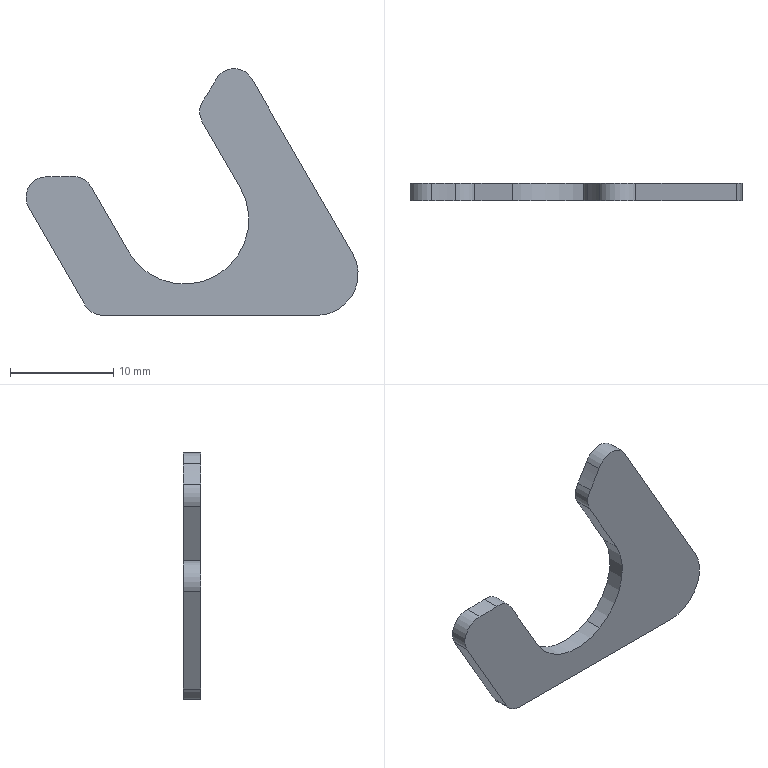Part | SolidWorks | features BaseBody 1 | 1 solid | 18 faces | box 32.238 x 1.7 x 23.947 mm | volume 539.449 mm3 | cylinder 11 | plane 7 | commonest cylinder face diameters 4 x5 8 x2 12.5 x2 35 x2
STEP:
#1=CARTESIAN_POINT('',(258.361,160.,-32.991));
#2=VERTEX_POINT('',#1);
#3=CARTESIAN_POINT('',(259.825,160.,-27.527));
#4=VERTEX_POINT('',#3);
#5=CARTESIAN_POINT('',(256.361,160.,-29.527));
#6=DIRECTION('',(0.,-1.,0.));
#7=DIRECTION('',(0.5,0.,-0.866));
#8=AXIS2_PLACEMENT_3D('',#5,#6,#7);
#9=CIRCLE('',#8,4.);
#10=EDGE_CURVE('',#2,#4,#9,.T.);
#11=ORIENTED_EDGE('',*,*,#10,.F.);
#12=CARTESIAN_POINT('',(258.361,161.7,-32.991));
#13=VERTEX_POINT('',#12);
#14=CARTESIAN_POINT('',(258.361,160.,-32.991));
#15=DIRECTION('',(0.,1.,0.));
#16=VECTOR('',#15,1000.);
#17=LINE('',#14,#16);
#18=EDGE_CURVE('',#2,#13,#17,.T.);
#19=ORIENTED_EDGE('',*,*,#18,.T.);
#20=CARTESIAN_POINT('',(259.825,161.7,-27.527));
#21=VERTEX_POINT('',#20);
#22=CARTESIAN_POINT('',(256.361,161.7,-29.527));
#23=DIRECTION('',(0.,-1.,0.));
#24=DIRECTION('',(0.5,0.,-0.866));
#25=AXIS2_PLACEMENT_3D('',#22,#23,#24);
#26=CIRCLE('',#25,4.);
#27=EDGE_CURVE('',#13,#21,#26,.T.);
#28=ORIENTED_EDGE('',*,*,#27,.T.);
#29=CARTESIAN_POINT('',(259.825,160.,-27.527));
#30=DIRECTION('',(0.,1.,0.));
#31=VECTOR('',#30,1000.);
#32=LINE('',#29,#31);
#33=EDGE_CURVE('',#4,#21,#32,.T.);
#34=ORIENTED_EDGE('',*,*,#33,.F.);
#35=EDGE_LOOP('',(#11,#19,#28,#34));
#36=FACE_OUTER_BOUND('',#35,.T.);
#37=CARTESIAN_POINT('',(256.361,160.,-29.527));
#38=DIRECTION('',(0.,1.,0.));
#39=DIRECTION('',(0.5,0.,-0.866));
#40=AXIS2_PLACEMENT_3D('',#37,#38,#39);
#41=CYLINDRICAL_SURFACE('',#40,4.);
#42=ADVANCED_FACE('',(#36),#41,.T.);
#43=CARTESIAN_POINT('',(246.625,160.,-29.663));
#44=VERTEX_POINT('',#43);
#45=CARTESIAN_POINT('',(238.087,160.,-27.375));
#46=VERTEX_POINT('',#45);
#47=CARTESIAN_POINT('',(243.5,160.,-24.25));
#48=DIRECTION('',(0.,1.,0.));
#49=DIRECTION('',(-0.5,0.,0.866));
#50=AXIS2_PLACEMENT_3D('',#47,#48,#49);
#51=CIRCLE('',#50,6.25);
#52=EDGE_CURVE('',#44,#46,#51,.T.);
#53=ORIENTED_EDGE('',*,*,#52,.F.);
#54=CARTESIAN_POINT('',(246.625,161.7,-29.663));
#55=VERTEX_POINT('',#54);
#56=CARTESIAN_POINT('',(246.625,160.,-29.663));
#57=DIRECTION('',(0.,1.,0.));
#58=VECTOR('',#57,1000.);
#59=LINE('',#56,#58);
#60=EDGE_CURVE('',#44,#55,#59,.T.);
#61=ORIENTED_EDGE('',*,*,#60,.T.);
#62=CARTESIAN_POINT('',(238.087,161.7,-27.375));
#63=VERTEX_POINT('',#62);
#64=CARTESIAN_POINT('',(243.5,161.7,-24.25));
#65=DIRECTION('',(0.,1.,0.));
#66=DIRECTION('',(-0.5,0.,0.866));
#67=AXIS2_PLACEMENT_3D('',#64,#65,#66);
#68=CIRCLE('',#67,6.25);
#69=EDGE_CURVE('',#55,#63,#68,.T.);
#70=ORIENTED_EDGE('',*,*,#69,.T.);
#71=CARTESIAN_POINT('',(238.087,160.,-27.375));
#72=DIRECTION('',(0.,1.,0.));
#73=VECTOR('',#72,1000.);
#74=LINE('',#71,#73);
#75=EDGE_CURVE('',#46,#63,#74,.T.);
#76=ORIENTED_EDGE('',*,*,#75,.F.);
#77=EDGE_LOOP('',(#53,#61,#70,#76));
#78=FACE_OUTER_BOUND('',#77,.T.);
#79=CARTESIAN_POINT('',(243.5,160.,-24.25));
#80=DIRECTION('',(0.,1.,0.));
#81=DIRECTION('',(0.5,0.,-0.866));
#82=AXIS2_PLACEMENT_3D('',#79,#80,#81);
#83=CYLINDRICAL_SURFACE('',#82,6.25);
#84=ADVANCED_FACE('',(#78),#83,.F.);
#85=ORIENTED_EDGE('',*,*,#60,.F.);
#86=CARTESIAN_POINT('',(248.913,160.,-21.125));
#87=VERTEX_POINT('',#86);
#88=CARTESIAN_POINT('',(243.5,160.,-24.25));
#89=DIRECTION('',(0.,1.,0.));
#90=DIRECTION('',(-0.5,0.,0.866));
#91=AXIS2_PLACEMENT_3D('',#88,#89,#90);
#92=CIRCLE('',#91,6.25);
#93=EDGE_CURVE('',#87,#44,#92,.T.);
#94=ORIENTED_EDGE('',*,*,#93,.F.);
#95=CARTESIAN_POINT('',(248.913,161.7,-21.125));
#96=VERTEX_POINT('',#95);
#97=CARTESIAN_POINT('',(248.913,160.,-21.125));
#98=DIRECTION('',(0.,1.,0.));
#99=VECTOR('',#98,1000.);
#100=LINE('',#97,#99);
#101=EDGE_CURVE('',#87,#96,#100,.T.);
#102=ORIENTED_EDGE('',*,*,#101,.T.);
#103=CARTESIAN_POINT('',(243.5,161.7,-24.25));
#104=DIRECTION('',(0.,1.,0.));
#105=DIRECTION('',(-0.5,0.,0.866));
#106=AXIS2_PLACEMENT_3D('',#103,#104,#105);
#107=CIRCLE('',#106,6.25);
#108=EDGE_CURVE('',#96,#55,#107,.T.);
#109=ORIENTED_EDGE('',*,*,#108,.T.);
#110=EDGE_LOOP('',(#85,#94,#102,#109));
#111=FACE_OUTER_BOUND('',#110,.T.);
#112=CARTESIAN_POINT('',(243.5,160.,-24.25));
#113=DIRECTION('',(0.,1.,0.));
#114=DIRECTION('',(0.5,0.,-0.866));
#115=AXIS2_PLACEMENT_3D('',#112,#113,#114);
#116=CYLINDRICAL_SURFACE('',#115,6.25);
#117=ADVANCED_FACE('',(#111),#116,.F.);
#118=CARTESIAN_POINT('',(234.422,161.7,-21.026));
#119=VERTEX_POINT('',#118);
#120=CARTESIAN_POINT('',(238.087,161.7,-27.375));
#121=DIRECTION('',(-0.5,0.,0.866));
#122=VECTOR('',#121,1000.);
#123=LINE('',#120,#122);
#124=EDGE_CURVE('',#63,#119,#123,.T.);
#125=ORIENTED_EDGE('',*,*,#124,.T.);
#126=CARTESIAN_POINT('',(234.422,160.,-21.026));
#127=VERTEX_POINT('',#126);
#128=CARTESIAN_POINT('',(234.422,160.,-21.026));
#129=DIRECTION('',(0.,1.,0.));
#130=VECTOR('',#129,1000.);
#131=LINE('',#128,#130);
#132=EDGE_CURVE('',#127,#119,#131,.T.);
#133=ORIENTED_EDGE('',*,*,#132,.F.);
#134=CARTESIAN_POINT('',(238.087,160.,-27.375));
#135=DIRECTION('',(-0.5,0.,0.866));
#136=VECTOR('',#135,1000.);
#137=LINE('',#134,#136);
#138=EDGE_CURVE('',#46,#127,#137,.T.);
#139=ORIENTED_EDGE('',*,*,#138,.F.);
#140=ORIENTED_EDGE('',*,*,#75,.T.);
#141=EDGE_LOOP('',(#125,#133,#139,#140));
#142=FACE_OUTER_BOUND('',#141,.T.);
#143=CARTESIAN_POINT('',(238.087,160.,-27.375));
#144=DIRECTION('',(-0.866,0.,-0.5));
#145=DIRECTION('',(0.5,0.,-0.866));
#146=AXIS2_PLACEMENT_3D('',#143,#144,#145);
#147=PLANE('',#146);
#148=ADVANCED_FACE('',(#142),#147,.F.);
#149=CARTESIAN_POINT('',(232.516,161.7,-20.033));
#150=VERTEX_POINT('',#149);
#151=CARTESIAN_POINT('',(232.69,161.7,-22.026));
#152=DIRECTION('',(0.,-1.,0.));
#153=DIRECTION('',(-0.5,0.,0.866));
#154=AXIS2_PLACEMENT_3D('',#151,#152,#153);
#155=CIRCLE('',#154,2.);
#156=EDGE_CURVE('',#119,#150,#155,.T.);
#157=ORIENTED_EDGE('',*,*,#156,.T.);
#158=CARTESIAN_POINT('',(232.516,160.,-20.033));
#159=VERTEX_POINT('',#158);
#160=CARTESIAN_POINT('',(232.516,160.,-20.033));
#161=DIRECTION('',(0.,1.,0.));
#162=VECTOR('',#161,1000.);
#163=LINE('',#160,#162);
#164=EDGE_CURVE('',#159,#150,#163,.T.);
#165=ORIENTED_EDGE('',*,*,#164,.F.);
#166=CARTESIAN_POINT('',(232.69,160.,-22.026));
#167=DIRECTION('',(0.,-1.,0.));
#168=DIRECTION('',(-0.5,0.,0.866));
#169=AXIS2_PLACEMENT_3D('',#166,#167,#168);
#170=CIRCLE('',#169,2.);
#171=EDGE_CURVE('',#127,#159,#170,.T.);
#172=ORIENTED_EDGE('',*,*,#171,.F.);
#173=ORIENTED_EDGE('',*,*,#132,.T.);
#174=EDGE_LOOP('',(#157,#165,#172,#173));
#175=FACE_OUTER_BOUND('',#174,.T.);
#176=CARTESIAN_POINT('',(232.69,160.,-22.026));
#177=DIRECTION('',(0.,1.,0.));
#178=DIRECTION('',(0.5,0.,-0.866));
#179=AXIS2_PLACEMENT_3D('',#176,#177,#178);
#180=CYLINDRICAL_SURFACE('',#179,2.);
#181=ADVANCED_FACE('',(#175),#180,.T.);
#182=CARTESIAN_POINT('',(230.213,161.7,-20.081));
#183=VERTEX_POINT('',#182);
#184=CARTESIAN_POINT('',(231.,161.7,-2.599));
#185=DIRECTION('',(0.,1.,0.));
#186=DIRECTION('',(-0.5,0.,0.866));
#187=AXIS2_PLACEMENT_3D('',#184,#185,#186);
#188=CIRCLE('',#187,17.5);
#189=EDGE_CURVE('',#150,#183,#188,.T.);
#190=ORIENTED_EDGE('',*,*,#189,.T.);
#191=CARTESIAN_POINT('',(230.213,160.,-20.081));
#192=VERTEX_POINT('',#191);
#193=CARTESIAN_POINT('',(230.213,160.,-20.081));
#194=DIRECTION('',(0.,1.,0.));
#195=VECTOR('',#194,1000.);
#196=LINE('',#193,#195);
#197=EDGE_CURVE('',#192,#183,#196,.T.);
#198=ORIENTED_EDGE('',*,*,#197,.F.);
#199=CARTESIAN_POINT('',(231.,160.,-2.599));
#200=DIRECTION('',(0.,1.,0.));
#201=DIRECTION('',(-0.5,0.,0.866));
#202=AXIS2_PLACEMENT_3D('',#199,#200,#201);
#203=CIRCLE('',#202,17.5);
#204=EDGE_CURVE('',#159,#192,#203,.T.);
#205=ORIENTED_EDGE('',*,*,#204,.F.);
#206=ORIENTED_EDGE('',*,*,#164,.T.);
#207=EDGE_LOOP('',(#190,#198,#205,#206));
#208=FACE_OUTER_BOUND('',#207,.T.);
#209=CARTESIAN_POINT('',(231.,160.,-2.599));
#210=DIRECTION('',(0.,1.,0.));
#211=DIRECTION('',(0.5,0.,-0.866));
#212=AXIS2_PLACEMENT_3D('',#209,#210,#211);
#213=CYLINDRICAL_SURFACE('',#212,17.5);
#214=ADVANCED_FACE('',(#208),#213,.F.);
#215=CARTESIAN_POINT('',(228.391,161.7,-23.079));
#216=VERTEX_POINT('',#215);
#217=CARTESIAN_POINT('',(230.123,161.7,-22.079));
#218=DIRECTION('',(0.,-1.,0.));
#219=DIRECTION('',(0.5,0.,-0.866));
#220=AXIS2_PLACEMENT_3D('',#217,#218,#219);
#221=CIRCLE('',#220,2.);
#222=EDGE_CURVE('',#183,#216,#221,.T.);
#223=ORIENTED_EDGE('',*,*,#222,.T.);
#224=CARTESIAN_POINT('',(228.391,160.,-23.079));
#225=VERTEX_POINT('',#224);
#226=CARTESIAN_POINT('',(228.391,160.,-23.079));
#227=DIRECTION('',(0.,1.,0.));
#228=VECTOR('',#227,1000.);
#229=LINE('',#226,#228);
#230=EDGE_CURVE('',#225,#216,#229,.T.);
#231=ORIENTED_EDGE('',*,*,#230,.F.);
#232=CARTESIAN_POINT('',(230.123,160.,-22.079));
#233=DIRECTION('',(0.,-1.,0.));
#234=DIRECTION('',(0.5,0.,-0.866));
#235=AXIS2_PLACEMENT_3D('',#232,#233,#234);
#236=CIRCLE('',#235,2.);
#237=EDGE_CURVE('',#192,#225,#236,.T.);
#238=ORIENTED_EDGE('',*,*,#237,.F.);
#239=ORIENTED_EDGE('',*,*,#197,.T.);
#240=EDGE_LOOP('',(#223,#231,#238,#239));
#241=FACE_OUTER_BOUND('',#240,.T.);
#242=CARTESIAN_POINT('',(230.123,160.,-22.079));
#243=DIRECTION('',(0.,1.,0.));
#244=DIRECTION('',(0.5,0.,-0.866));
#245=AXIS2_PLACEMENT_3D('',#242,#243,#244);
#246=CYLINDRICAL_SURFACE('',#245,2.);
#247=ADVANCED_FACE('',(#241),#246,.T.);
#248=CARTESIAN_POINT('',(233.844,161.7,-32.526));
#249=VERTEX_POINT('',#248);
#250=CARTESIAN_POINT('',(233.844,161.7,-32.526));
#251=DIRECTION('',(0.5,0.,-0.866));
#252=VECTOR('',#251,1000.);
#253=LINE('',#250,#252);
#254=EDGE_CURVE('',#216,#249,#253,.T.);
#255=ORIENTED_EDGE('',*,*,#254,.T.);
#256=CARTESIAN_POINT('',(233.844,160.,-32.526));
#257=VERTEX_POINT('',#256);
#258=CARTESIAN_POINT('',(233.844,160.,-32.526));
#259=DIRECTION('',(0.,1.,0.));
#260=VECTOR('',#259,1000.);
#261=LINE('',#258,#260);
#262=EDGE_CURVE('',#257,#249,#261,.T.);
#263=ORIENTED_EDGE('',*,*,#262,.F.);
#264=CARTESIAN_POINT('',(233.844,160.,-32.526));
#265=DIRECTION('',(0.5,0.,-0.866));
#266=VECTOR('',#265,1000.);
#267=LINE('',#264,#266);
#268=EDGE_CURVE('',#225,#257,#267,.T.);
#269=ORIENTED_EDGE('',*,*,#268,.F.);
#270=ORIENTED_EDGE('',*,*,#230,.T.);
#271=EDGE_LOOP('',(#255,#263,#269,#270));
#272=FACE_OUTER_BOUND('',#271,.T.);
#273=CARTESIAN_POINT('',(233.844,160.,-32.526));
#274=DIRECTION('',(0.866,0.,0.5));
#275=DIRECTION('',(-0.5,0.,0.866));
#276=AXIS2_PLACEMENT_3D('',#273,#274,#275);
#277=PLANE('',#276);
#278=ADVANCED_FACE('',(#272),#277,.F.);
#279=CARTESIAN_POINT('',(235.576,161.7,-33.526));
#280=VERTEX_POINT('',#279);
#281=CARTESIAN_POINT('',(235.576,161.7,-31.526));
#282=DIRECTION('',(0.,-1.,0.));
#283=DIRECTION('',(0.5,0.,-0.866));
#284=AXIS2_PLACEMENT_3D('',#281,#282,#283);
#285=CIRCLE('',#284,2.);
#286=EDGE_CURVE('',#249,#280,#285,.T.);
#287=ORIENTED_EDGE('',*,*,#286,.T.);
#288=CARTESIAN_POINT('',(235.576,160.,-33.526));
#289=VERTEX_POINT('',#288);
#290=CARTESIAN_POINT('',(235.576,160.,-33.526));
#291=DIRECTION('',(0.,1.,0.));
#292=VECTOR('',#291,1000.);
#293=LINE('',#290,#292);
#294=EDGE_CURVE('',#289,#280,#293,.T.);
#295=ORIENTED_EDGE('',*,*,#294,.F.);
#296=CARTESIAN_POINT('',(235.576,160.,-31.526));
#297=DIRECTION('',(0.,-1.,0.));
#298=DIRECTION('',(0.5,0.,-0.866));
#299=AXIS2_PLACEMENT_3D('',#296,#297,#298);
#300=CIRCLE('',#299,2.);
#301=EDGE_CURVE('',#257,#289,#300,.T.);
#302=ORIENTED_EDGE('',*,*,#301,.F.);
#303=ORIENTED_EDGE('',*,*,#262,.T.);
#304=EDGE_LOOP('',(#287,#295,#302,#303));
#305=FACE_OUTER_BOUND('',#304,.T.);
#306=CARTESIAN_POINT('',(235.576,160.,-31.526));
#307=DIRECTION('',(0.,1.,0.));
#308=DIRECTION('',(0.5,0.,-0.866));
#309=AXIS2_PLACEMENT_3D('',#306,#307,#308);
#310=CYLINDRICAL_SURFACE('',#309,2.);
#311=ADVANCED_FACE('',(#305),#310,.T.);
#312=CARTESIAN_POINT('',(256.361,161.7,-33.527));
#313=VERTEX_POINT('',#312);
#314=CARTESIAN_POINT('',(235.576,161.7,-33.526));
#315=DIRECTION('',(1.,0.,-0.00002301));
#316=VECTOR('',#315,1000.);
#317=LINE('',#314,#316);
#318=EDGE_CURVE('',#280,#313,#317,.T.);
#319=ORIENTED_EDGE('',*,*,#318,.T.);
#320=CARTESIAN_POINT('',(256.361,160.,-33.527));
#321=VERTEX_POINT('',#320);
#322=CARTESIAN_POINT('',(256.361,160.,-33.527));
#323=DIRECTION('',(0.,1.,0.));
#324=VECTOR('',#323,1000.);
#325=LINE('',#322,#324);
#326=EDGE_CURVE('',#321,#313,#325,.T.);
#327=ORIENTED_EDGE('',*,*,#326,.F.);
#328=CARTESIAN_POINT('',(235.576,160.,-33.526));
#329=DIRECTION('',(1.,0.,-0.00002301));
#330=VECTOR('',#329,1000.);
#331=LINE('',#328,#330);
#332=EDGE_CURVE('',#289,#321,#331,.T.);
#333=ORIENTED_EDGE('',*,*,#332,.F.);
#334=ORIENTED_EDGE('',*,*,#294,.T.);
#335=EDGE_LOOP('',(#319,#327,#333,#334));
#336=FACE_OUTER_BOUND('',#335,.T.);
#337=CARTESIAN_POINT('',(235.576,160.,-33.526));
#338=DIRECTION('',(0.00002301,0.,1.));
#339=DIRECTION('',(-1.,0.,0.00002301));
#340=AXIS2_PLACEMENT_3D('',#337,#338,#339);
#341=PLANE('',#340);
#342=ADVANCED_FACE('',(#336),#341,.F.);
#343=ORIENTED_EDGE('',*,*,#18,.F.);
#344=CARTESIAN_POINT('',(256.361,160.,-29.527));
#345=DIRECTION('',(0.,-1.,0.));
#346=DIRECTION('',(0.5,0.,-0.866));
#347=AXIS2_PLACEMENT_3D('',#344,#345,#346);
#348=CIRCLE('',#347,4.);
#349=EDGE_CURVE('',#321,#2,#348,.T.);
#350=ORIENTED_EDGE('',*,*,#349,.F.);
#351=ORIENTED_EDGE('',*,*,#326,.T.);
#352=CARTESIAN_POINT('',(256.361,161.7,-29.527));
#353=DIRECTION('',(0.,-1.,0.));
#354=DIRECTION('',(0.5,0.,-0.866));
#355=AXIS2_PLACEMENT_3D('',#352,#353,#354);
#356=CIRCLE('',#355,4.);
#357=EDGE_CURVE('',#313,#13,#356,.T.);
#358=ORIENTED_EDGE('',*,*,#357,.T.);
#359=EDGE_LOOP('',(#343,#350,#351,#358));
#360=FACE_OUTER_BOUND('',#359,.T.);
#361=CARTESIAN_POINT('',(256.361,160.,-29.527));
#362=DIRECTION('',(0.,1.,0.));
#363=DIRECTION('',(0.5,0.,-0.866));
#364=AXIS2_PLACEMENT_3D('',#361,#362,#363);
#365=CYLINDRICAL_SURFACE('',#364,4.);
#366=ADVANCED_FACE('',(#360),#365,.T.);
#367=CARTESIAN_POINT('',(250.041,161.7,-10.58));
#368=VERTEX_POINT('',#367);
#369=CARTESIAN_POINT('',(259.825,161.7,-27.527));
#370=DIRECTION('',(-0.5,0.,0.866));
#371=VECTOR('',#370,1000.);
#372=LINE('',#369,#371);
#373=EDGE_CURVE('',#21,#368,#372,.T.);
#374=ORIENTED_EDGE('',*,*,#373,.T.);
#375=CARTESIAN_POINT('',(250.041,160.,-10.58));
#376=VERTEX_POINT('',#375);
#377=CARTESIAN_POINT('',(250.041,160.,-10.58));
#378=DIRECTION('',(0.,1.,0.));
#379=VECTOR('',#378,1000.);
#380=LINE('',#377,#379);
#381=EDGE_CURVE('',#376,#368,#380,.T.);
#382=ORIENTED_EDGE('',*,*,#381,.F.);
#383=CARTESIAN_POINT('',(259.825,160.,-27.527));
#384=DIRECTION('',(-0.5,0.,0.866));
#385=VECTOR('',#384,1000.);
#386=LINE('',#383,#385);
#387=EDGE_CURVE('',#4,#376,#386,.T.);
#388=ORIENTED_EDGE('',*,*,#387,.F.);
#389=ORIENTED_EDGE('',*,*,#33,.T.);
#390=EDGE_LOOP('',(#374,#382,#388,#389));
#391=FACE_OUTER_BOUND('',#390,.T.);
#392=CARTESIAN_POINT('',(259.825,160.,-27.527));
#393=DIRECTION('',(-0.866,0.,-0.5));
#394=DIRECTION('',(0.5,0.,-0.866));
#395=AXIS2_PLACEMENT_3D('',#392,#393,#394);
#396=PLANE('',#395);
#397=ADVANCED_FACE('',(#391),#396,.F.);
#398=CARTESIAN_POINT('',(246.534,161.7,-10.659));
#399=VERTEX_POINT('',#398);
#400=CARTESIAN_POINT('',(248.309,161.7,-11.58));
#401=DIRECTION('',(0.,-1.,0.));
#402=DIRECTION('',(-0.5,0.,0.866));
#403=AXIS2_PLACEMENT_3D('',#400,#401,#402);
#404=CIRCLE('',#403,2.);
#405=EDGE_CURVE('',#368,#399,#404,.T.);
#406=ORIENTED_EDGE('',*,*,#405,.T.);
#407=CARTESIAN_POINT('',(246.534,160.,-10.659));
#408=VERTEX_POINT('',#407);
#409=CARTESIAN_POINT('',(246.534,160.,-10.659));
#410=DIRECTION('',(0.,1.,0.));
#411=VECTOR('',#410,1000.);
#412=LINE('',#409,#411);
#413=EDGE_CURVE('',#408,#399,#412,.T.);
#414=ORIENTED_EDGE('',*,*,#413,.F.);
#415=CARTESIAN_POINT('',(248.309,160.,-11.58));
#416=DIRECTION('',(0.,-1.,0.));
#417=DIRECTION('',(-0.5,0.,0.866));
#418=AXIS2_PLACEMENT_3D('',#415,#416,#417);
#419=CIRCLE('',#418,2.);
#420=EDGE_CURVE('',#376,#408,#419,.T.);
#421=ORIENTED_EDGE('',*,*,#420,.F.);
#422=ORIENTED_EDGE('',*,*,#381,.T.);
#423=EDGE_LOOP('',(#406,#414,#421,#422));
#424=FACE_OUTER_BOUND('',#423,.T.);
#425=CARTESIAN_POINT('',(248.309,160.,-11.58));
#426=DIRECTION('',(0.,1.,0.));
#427=DIRECTION('',(0.5,0.,-0.866));
#428=AXIS2_PLACEMENT_3D('',#425,#426,#427);
#429=CYLINDRICAL_SURFACE('',#428,2.);
#430=ADVANCED_FACE('',(#424),#429,.T.);
#431=CARTESIAN_POINT('',(245.341,161.7,-12.63));
#432=VERTEX_POINT('',#431);
#433=CARTESIAN_POINT('',(231.,161.7,-2.599));
#434=DIRECTION('',(0.,1.,0.));
#435=DIRECTION('',(-0.5,0.,0.866));
#436=AXIS2_PLACEMENT_3D('',#433,#434,#435);
#437=CIRCLE('',#436,17.5);
#438=EDGE_CURVE('',#399,#432,#437,.T.);
#439=ORIENTED_EDGE('',*,*,#438,.T.);
#440=CARTESIAN_POINT('',(245.341,160.,-12.63));
#441=VERTEX_POINT('',#440);
#442=CARTESIAN_POINT('',(245.341,160.,-12.63));
#443=DIRECTION('',(0.,1.,0.));
#444=VECTOR('',#443,1000.);
#445=LINE('',#442,#444);
#446=EDGE_CURVE('',#441,#432,#445,.T.);
#447=ORIENTED_EDGE('',*,*,#446,.F.);
#448=CARTESIAN_POINT('',(231.,160.,-2.599));
#449=DIRECTION('',(0.,1.,0.));
#450=DIRECTION('',(-0.5,0.,0.866));
#451=AXIS2_PLACEMENT_3D('',#448,#449,#450);
#452=CIRCLE('',#451,17.5);
#453=EDGE_CURVE('',#408,#441,#452,.T.);
#454=ORIENTED_EDGE('',*,*,#453,.F.);
#455=ORIENTED_EDGE('',*,*,#413,.T.);
#456=EDGE_LOOP('',(#439,#447,#454,#455));
#457=FACE_OUTER_BOUND('',#456,.T.);
#458=CARTESIAN_POINT('',(231.,160.,-2.599));
#459=DIRECTION('',(0.,1.,0.));
#460=DIRECTION('',(0.5,0.,-0.866));
#461=AXIS2_PLACEMENT_3D('',#458,#459,#460);
#462=CYLINDRICAL_SURFACE('',#461,17.5);
#463=ADVANCED_FACE('',(#457),#462,.F.);
#464=CARTESIAN_POINT('',(245.247,161.7,-14.776));
#465=VERTEX_POINT('',#464);
#466=CARTESIAN_POINT('',(246.979,161.7,-13.776));
#467=DIRECTION('',(0.,-1.,0.));
#468=DIRECTION('',(0.5,0.,-0.866));
#469=AXIS2_PLACEMENT_3D('',#466,#467,#468);
#470=CIRCLE('',#469,2.);
#471=EDGE_CURVE('',#432,#465,#470,.T.);
#472=ORIENTED_EDGE('',*,*,#471,.T.);
#473=CARTESIAN_POINT('',(245.247,160.,-14.776));
#474=VERTEX_POINT('',#473);
#475=CARTESIAN_POINT('',(245.247,160.,-14.776));
#476=DIRECTION('',(0.,1.,0.));
#477=VECTOR('',#476,1000.);
#478=LINE('',#475,#477);
#479=EDGE_CURVE('',#474,#465,#478,.T.);
#480=ORIENTED_EDGE('',*,*,#479,.F.);
#481=CARTESIAN_POINT('',(246.979,160.,-13.776));
#482=DIRECTION('',(0.,-1.,0.));
#483=DIRECTION('',(0.5,0.,-0.866));
#484=AXIS2_PLACEMENT_3D('',#481,#482,#483);
#485=CIRCLE('',#484,2.);
#486=EDGE_CURVE('',#441,#474,#485,.T.);
#487=ORIENTED_EDGE('',*,*,#486,.F.);
#488=ORIENTED_EDGE('',*,*,#446,.T.);
#489=EDGE_LOOP('',(#472,#480,#487,#488));
#490=FACE_OUTER_BOUND('',#489,.T.);
#491=CARTESIAN_POINT('',(246.979,160.,-13.776));
#492=DIRECTION('',(0.,1.,0.));
#493=DIRECTION('',(0.5,0.,-0.866));
#494=AXIS2_PLACEMENT_3D('',#491,#492,#493);
#495=CYLINDRICAL_SURFACE('',#494,2.);
#496=ADVANCED_FACE('',(#490),#495,.T.);
#497=CARTESIAN_POINT('',(248.913,161.7,-21.125));
#498=DIRECTION('',(0.5,0.,-0.866));
#499=VECTOR('',#498,1000.);
#500=LINE('',#497,#499);
#501=EDGE_CURVE('',#465,#96,#500,.T.);
#502=ORIENTED_EDGE('',*,*,#501,.T.);
#503=ORIENTED_EDGE('',*,*,#101,.F.);
#504=CARTESIAN_POINT('',(248.913,160.,-21.125));
#505=DIRECTION('',(0.5,0.,-0.866));
#506=VECTOR('',#505,1000.);
#507=LINE('',#504,#506);
#508=EDGE_CURVE('',#474,#87,#507,.T.);
#509=ORIENTED_EDGE('',*,*,#508,.F.);
#510=ORIENTED_EDGE('',*,*,#479,.T.);
#511=EDGE_LOOP('',(#502,#503,#509,#510));
#512=FACE_OUTER_BOUND('',#511,.T.);
#513=CARTESIAN_POINT('',(248.913,160.,-21.125));
#514=DIRECTION('',(0.866,0.,0.5));
#515=DIRECTION('',(-0.5,0.,0.866));
#516=AXIS2_PLACEMENT_3D('',#513,#514,#515);
#517=PLANE('',#516);
#518=ADVANCED_FACE('',(#512),#517,.F.);
#519=ORIENTED_EDGE('',*,*,#93,.T.);
#520=ORIENTED_EDGE('',*,*,#52,.T.);
#521=ORIENTED_EDGE('',*,*,#138,.T.);
#522=ORIENTED_EDGE('',*,*,#171,.T.);
#523=ORIENTED_EDGE('',*,*,#204,.T.);
#524=ORIENTED_EDGE('',*,*,#237,.T.);
#525=ORIENTED_EDGE('',*,*,#268,.T.);
#526=ORIENTED_EDGE('',*,*,#301,.T.);
#527=ORIENTED_EDGE('',*,*,#332,.T.);
#528=ORIENTED_EDGE('',*,*,#349,.T.);
#529=ORIENTED_EDGE('',*,*,#10,.T.);
#530=ORIENTED_EDGE('',*,*,#387,.T.);
#531=ORIENTED_EDGE('',*,*,#420,.T.);
#532=ORIENTED_EDGE('',*,*,#453,.T.);
#533=ORIENTED_EDGE('',*,*,#486,.T.);
#534=ORIENTED_EDGE('',*,*,#508,.T.);
#535=EDGE_LOOP('',(#519,#520,#521,#522,#523,#524,#525,#526,#527,#528,#529,#530,#531,#532,#533,#534));
#536=FACE_OUTER_BOUND('',#535,.T.);
#537=CARTESIAN_POINT('',(243.5,160.,-24.25));
#538=DIRECTION('',(0.,-1.,0.));
#539=DIRECTION('',(-0.5,0.,0.866));
#540=AXIS2_PLACEMENT_3D('',#537,#538,#539);
#541=PLANE('',#540);
#542=ADVANCED_FACE('',(#536),#541,.T.);
#543=ORIENTED_EDGE('',*,*,#108,.F.);
#544=ORIENTED_EDGE('',*,*,#501,.F.);
#545=ORIENTED_EDGE('',*,*,#471,.F.);
#546=ORIENTED_EDGE('',*,*,#438,.F.);
#547=ORIENTED_EDGE('',*,*,#405,.F.);
#548=ORIENTED_EDGE('',*,*,#373,.F.);
#549=ORIENTED_EDGE('',*,*,#27,.F.);
#550=ORIENTED_EDGE('',*,*,#357,.F.);
#551=ORIENTED_EDGE('',*,*,#318,.F.);
#552=ORIENTED_EDGE('',*,*,#286,.F.);
#553=ORIENTED_EDGE('',*,*,#254,.F.);
#554=ORIENTED_EDGE('',*,*,#222,.F.);
#555=ORIENTED_EDGE('',*,*,#189,.F.);
#556=ORIENTED_EDGE('',*,*,#156,.F.);
#557=ORIENTED_EDGE('',*,*,#124,.F.);
#558=ORIENTED_EDGE('',*,*,#69,.F.);
#559=EDGE_LOOP('',(#543,#544,#545,#546,#547,#548,#549,#550,#551,#552,#553,#554,#555,#556,#557,#558));
#560=FACE_OUTER_BOUND('',#559,.T.);
#561=CARTESIAN_POINT('',(243.5,161.7,-24.25));
#562=DIRECTION('',(0.,-1.,0.));
#563=DIRECTION('',(-0.5,0.,0.866));
#564=AXIS2_PLACEMENT_3D('',#561,#562,#563);
#565=PLANE('',#564);
#566=ADVANCED_FACE('',(#560),#565,.F.);
#567=CLOSED_SHELL('',(#42,#84,#117,#148,#181,#214,#247,#278,#311,#342,#366,#397,#430,#463,#496,#518,#542,#566));
#568=MANIFOLD_SOLID_BREP('',#567);
#569=CARTESIAN_POINT('',(0.,0.,0.));
#570=DIRECTION('',(0.,0.,1.));
#571=DIRECTION('',(1.,0.,0.));
#572=AXIS2_PLACEMENT_3D('',#569,#570,#571);
#573=(LENGTH_UNIT()NAMED_UNIT(*)SI_UNIT(.MILLI.,.METRE.));
#574=UNCERTAINTY_MEASURE_WITH_UNIT(LENGTH_MEASURE(0.00001),#573,'','');
#575=(NAMED_UNIT(*)PLANE_ANGLE_UNIT()SI_UNIT($,.RADIAN.));
#576=(NAMED_UNIT(*)SI_UNIT($,.STERADIAN.)SOLID_ANGLE_UNIT());
#577=(GEOMETRIC_REPRESENTATION_CONTEXT(3)GLOBAL_UNCERTAINTY_ASSIGNED_CONTEXT((#574))GLOBAL_UNIT_ASSIGNED_CONTEXT((#573,#575,#576))REPRESENTATION_CONTEXT('',''));
#578=ADVANCED_BREP_SHAPE_REPRESENTATION('',(#568,#572),#577);